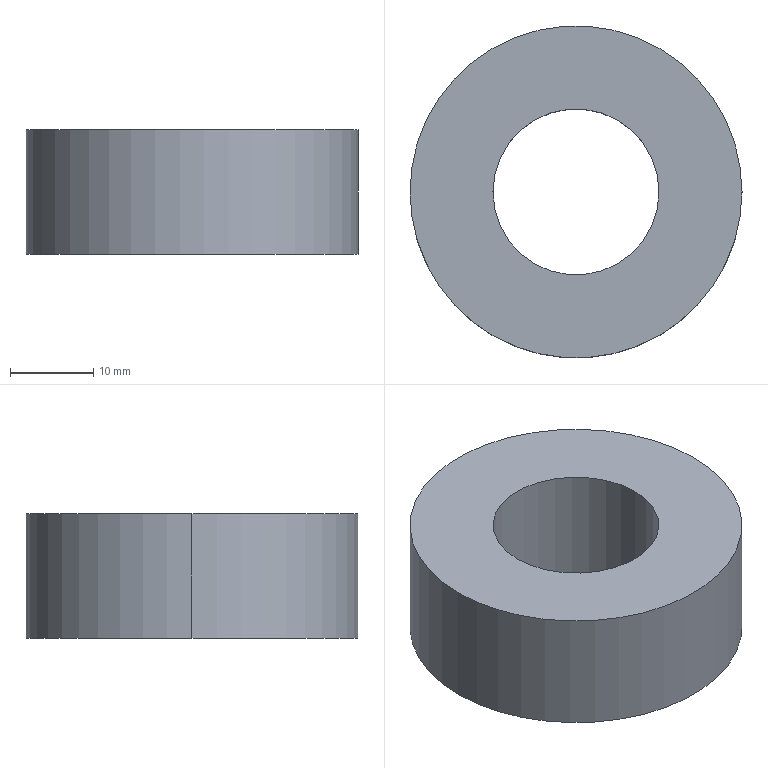Part | SolidWorks | features Extrusion 1 | 1 solid | 6 faces | box 40 x 40 x 15 mm | volume 14137 mm3 | cylinder 4 | plane 2 | commonest cylinder face diameters 20 x2 40 x2
STEP:
#1=CARTESIAN_POINT('',(-10.,0.,7.5));
#2=VERTEX_POINT('',#1);
#3=CARTESIAN_POINT('',(10.,0.,7.5));
#4=VERTEX_POINT('',#3);
#5=CARTESIAN_POINT('',(0.,0.,7.5));
#6=DIRECTION('',(0.,0.,1.));
#7=DIRECTION('',(1.,0.,0.));
#8=AXIS2_PLACEMENT_3D('',#5,#6,#7);
#9=CIRCLE('',#8,10.);
#10=EDGE_CURVE('',#2,#4,#9,.T.);
#11=ORIENTED_EDGE('',*,*,#10,.T.);
#12=CARTESIAN_POINT('',(10.,0.,-7.5));
#13=VERTEX_POINT('',#12);
#14=CARTESIAN_POINT('',(10.,0.,7.5));
#15=DIRECTION('',(0.,0.,-1.));
#16=VECTOR('',#15,1000.);
#17=LINE('',#14,#16);
#18=EDGE_CURVE('',#4,#13,#17,.T.);
#19=ORIENTED_EDGE('',*,*,#18,.T.);
#20=CARTESIAN_POINT('',(-10.,0.,-7.5));
#21=VERTEX_POINT('',#20);
#22=CARTESIAN_POINT('',(0.,0.,-7.5));
#23=DIRECTION('',(0.,0.,1.));
#24=DIRECTION('',(1.,0.,0.));
#25=AXIS2_PLACEMENT_3D('',#22,#23,#24);
#26=CIRCLE('',#25,10.);
#27=EDGE_CURVE('',#21,#13,#26,.T.);
#28=ORIENTED_EDGE('',*,*,#27,.F.);
#29=CARTESIAN_POINT('',(-10.,0.,7.5));
#30=DIRECTION('',(0.,0.,-1.));
#31=VECTOR('',#30,1000.);
#32=LINE('',#29,#31);
#33=EDGE_CURVE('',#2,#21,#32,.T.);
#34=ORIENTED_EDGE('',*,*,#33,.F.);
#35=EDGE_LOOP('',(#11,#19,#28,#34));
#36=FACE_OUTER_BOUND('',#35,.T.);
#37=CARTESIAN_POINT('',(0.,0.,7.5));
#38=DIRECTION('',(0.,0.,-1.));
#39=DIRECTION('',(-1.,0.,0.));
#40=AXIS2_PLACEMENT_3D('',#37,#38,#39);
#41=CYLINDRICAL_SURFACE('',#40,10.);
#42=ADVANCED_FACE('',(#36),#41,.F.);
#43=CARTESIAN_POINT('',(20.,0.,7.5));
#44=VERTEX_POINT('',#43);
#45=CARTESIAN_POINT('',(-20.,0.,7.5));
#46=VERTEX_POINT('',#45);
#47=CARTESIAN_POINT('',(0.,0.,7.5));
#48=DIRECTION('',(0.,0.,1.));
#49=DIRECTION('',(1.,0.,0.));
#50=AXIS2_PLACEMENT_3D('',#47,#48,#49);
#51=CIRCLE('',#50,20.);
#52=EDGE_CURVE('',#44,#46,#51,.T.);
#53=ORIENTED_EDGE('',*,*,#52,.F.);
#54=CARTESIAN_POINT('',(20.,0.,-7.5));
#55=VERTEX_POINT('',#54);
#56=CARTESIAN_POINT('',(20.,0.,7.5));
#57=DIRECTION('',(0.,0.,-1.));
#58=VECTOR('',#57,1000.);
#59=LINE('',#56,#58);
#60=EDGE_CURVE('',#44,#55,#59,.T.);
#61=ORIENTED_EDGE('',*,*,#60,.T.);
#62=CARTESIAN_POINT('',(-20.,0.,-7.5));
#63=VERTEX_POINT('',#62);
#64=CARTESIAN_POINT('',(0.,0.,-7.5));
#65=DIRECTION('',(0.,0.,1.));
#66=DIRECTION('',(1.,0.,0.));
#67=AXIS2_PLACEMENT_3D('',#64,#65,#66);
#68=CIRCLE('',#67,20.);
#69=EDGE_CURVE('',#55,#63,#68,.T.);
#70=ORIENTED_EDGE('',*,*,#69,.T.);
#71=CARTESIAN_POINT('',(-20.,0.,7.5));
#72=DIRECTION('',(0.,0.,-1.));
#73=VECTOR('',#72,1000.);
#74=LINE('',#71,#73);
#75=EDGE_CURVE('',#46,#63,#74,.T.);
#76=ORIENTED_EDGE('',*,*,#75,.F.);
#77=EDGE_LOOP('',(#53,#61,#70,#76));
#78=FACE_OUTER_BOUND('',#77,.T.);
#79=CARTESIAN_POINT('',(0.,0.,7.5));
#80=DIRECTION('',(0.,0.,-1.));
#81=DIRECTION('',(-1.,0.,0.));
#82=AXIS2_PLACEMENT_3D('',#79,#80,#81);
#83=CYLINDRICAL_SURFACE('',#82,20.);
#84=ADVANCED_FACE('',(#78),#83,.T.);
#85=CARTESIAN_POINT('',(0.,0.,7.5));
#86=DIRECTION('',(0.,0.,1.));
#87=DIRECTION('',(1.,0.,0.));
#88=AXIS2_PLACEMENT_3D('',#85,#86,#87);
#89=CIRCLE('',#88,20.);
#90=EDGE_CURVE('',#46,#44,#89,.T.);
#91=ORIENTED_EDGE('',*,*,#90,.T.);
#92=ORIENTED_EDGE('',*,*,#52,.T.);
#93=EDGE_LOOP('',(#91,#92));
#94=FACE_OUTER_BOUND('',#93,.T.);
#95=ORIENTED_EDGE('',*,*,#10,.F.);
#96=CARTESIAN_POINT('',(0.,0.,7.5));
#97=DIRECTION('',(0.,0.,1.));
#98=DIRECTION('',(1.,0.,0.));
#99=AXIS2_PLACEMENT_3D('',#96,#97,#98);
#100=CIRCLE('',#99,10.);
#101=EDGE_CURVE('',#4,#2,#100,.T.);
#102=ORIENTED_EDGE('',*,*,#101,.F.);
#103=EDGE_LOOP('',(#95,#102));
#104=FACE_BOUND('',#103,.T.);
#105=CARTESIAN_POINT('',(0.,0.,7.5));
#106=DIRECTION('',(0.,0.,1.));
#107=DIRECTION('',(1.,0.,0.));
#108=AXIS2_PLACEMENT_3D('',#105,#106,#107);
#109=PLANE('',#108);
#110=ADVANCED_FACE('',(#94,#104),#109,.T.);
#111=CARTESIAN_POINT('',(0.,0.,-7.5));
#112=DIRECTION('',(0.,0.,1.));
#113=DIRECTION('',(1.,0.,0.));
#114=AXIS2_PLACEMENT_3D('',#111,#112,#113);
#115=CIRCLE('',#114,20.);
#116=EDGE_CURVE('',#63,#55,#115,.T.);
#117=ORIENTED_EDGE('',*,*,#116,.F.);
#118=ORIENTED_EDGE('',*,*,#69,.F.);
#119=EDGE_LOOP('',(#117,#118));
#120=FACE_OUTER_BOUND('',#119,.T.);
#121=ORIENTED_EDGE('',*,*,#27,.T.);
#122=CARTESIAN_POINT('',(0.,0.,-7.5));
#123=DIRECTION('',(0.,0.,1.));
#124=DIRECTION('',(1.,0.,0.));
#125=AXIS2_PLACEMENT_3D('',#122,#123,#124);
#126=CIRCLE('',#125,10.);
#127=EDGE_CURVE('',#13,#21,#126,.T.);
#128=ORIENTED_EDGE('',*,*,#127,.T.);
#129=EDGE_LOOP('',(#121,#128));
#130=FACE_BOUND('',#129,.T.);
#131=CARTESIAN_POINT('',(0.,0.,-7.5));
#132=DIRECTION('',(0.,0.,1.));
#133=DIRECTION('',(1.,0.,0.));
#134=AXIS2_PLACEMENT_3D('',#131,#132,#133);
#135=PLANE('',#134);
#136=ADVANCED_FACE('',(#120,#130),#135,.F.);
#137=ORIENTED_EDGE('',*,*,#60,.F.);
#138=ORIENTED_EDGE('',*,*,#90,.F.);
#139=ORIENTED_EDGE('',*,*,#75,.T.);
#140=ORIENTED_EDGE('',*,*,#116,.T.);
#141=EDGE_LOOP('',(#137,#138,#139,#140));
#142=FACE_OUTER_BOUND('',#141,.T.);
#143=CARTESIAN_POINT('',(0.,0.,7.5));
#144=DIRECTION('',(0.,0.,-1.));
#145=DIRECTION('',(-1.,0.,0.));
#146=AXIS2_PLACEMENT_3D('',#143,#144,#145);
#147=CYLINDRICAL_SURFACE('',#146,20.);
#148=ADVANCED_FACE('',(#142),#147,.T.);
#149=ORIENTED_EDGE('',*,*,#18,.F.);
#150=ORIENTED_EDGE('',*,*,#101,.T.);
#151=ORIENTED_EDGE('',*,*,#33,.T.);
#152=ORIENTED_EDGE('',*,*,#127,.F.);
#153=EDGE_LOOP('',(#149,#150,#151,#152));
#154=FACE_OUTER_BOUND('',#153,.T.);
#155=CARTESIAN_POINT('',(0.,0.,7.5));
#156=DIRECTION('',(0.,0.,-1.));
#157=DIRECTION('',(-1.,0.,0.));
#158=AXIS2_PLACEMENT_3D('',#155,#156,#157);
#159=CYLINDRICAL_SURFACE('',#158,10.);
#160=ADVANCED_FACE('',(#154),#159,.F.);
#161=CLOSED_SHELL('',(#42,#84,#110,#136,#148,#160));
#162=MANIFOLD_SOLID_BREP('',#161);
#163=CARTESIAN_POINT('',(0.,0.,0.));
#164=DIRECTION('',(0.,0.,1.));
#165=DIRECTION('',(1.,0.,0.));
#166=AXIS2_PLACEMENT_3D('',#163,#164,#165);
#167=(LENGTH_UNIT()NAMED_UNIT(*)SI_UNIT(.MILLI.,.METRE.));
#168=UNCERTAINTY_MEASURE_WITH_UNIT(LENGTH_MEASURE(0.00001),#167,'','');
#169=(NAMED_UNIT(*)PLANE_ANGLE_UNIT()SI_UNIT($,.RADIAN.));
#170=(NAMED_UNIT(*)SI_UNIT($,.STERADIAN.)SOLID_ANGLE_UNIT());
#171=(GEOMETRIC_REPRESENTATION_CONTEXT(3)GLOBAL_UNCERTAINTY_ASSIGNED_CONTEXT((#168))GLOBAL_UNIT_ASSIGNED_CONTEXT((#167,#169,#170))REPRESENTATION_CONTEXT('',''));
#172=ADVANCED_BREP_SHAPE_REPRESENTATION('',(#162,#166),#171);